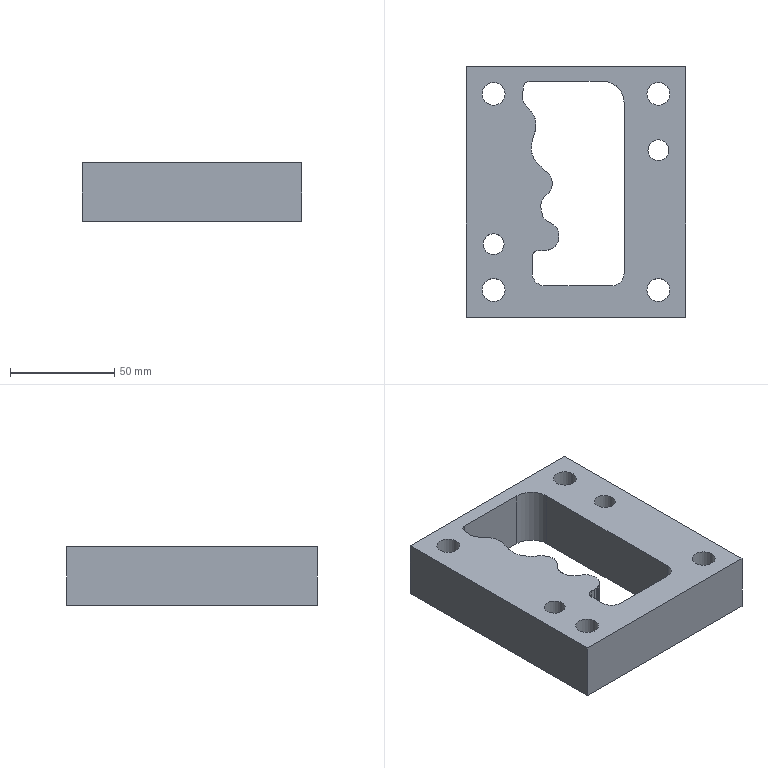Part | STEP file | PN_0020_id958_x_t | 1 solid | 144 faces | box 105 x 120 x 28 mm | volume 217134 mm3 | plane 127 | cylinder 17 | commonest cylinder face diameters 11 x4 12 x4 17 x4 6 x2 10 x2 20 x1